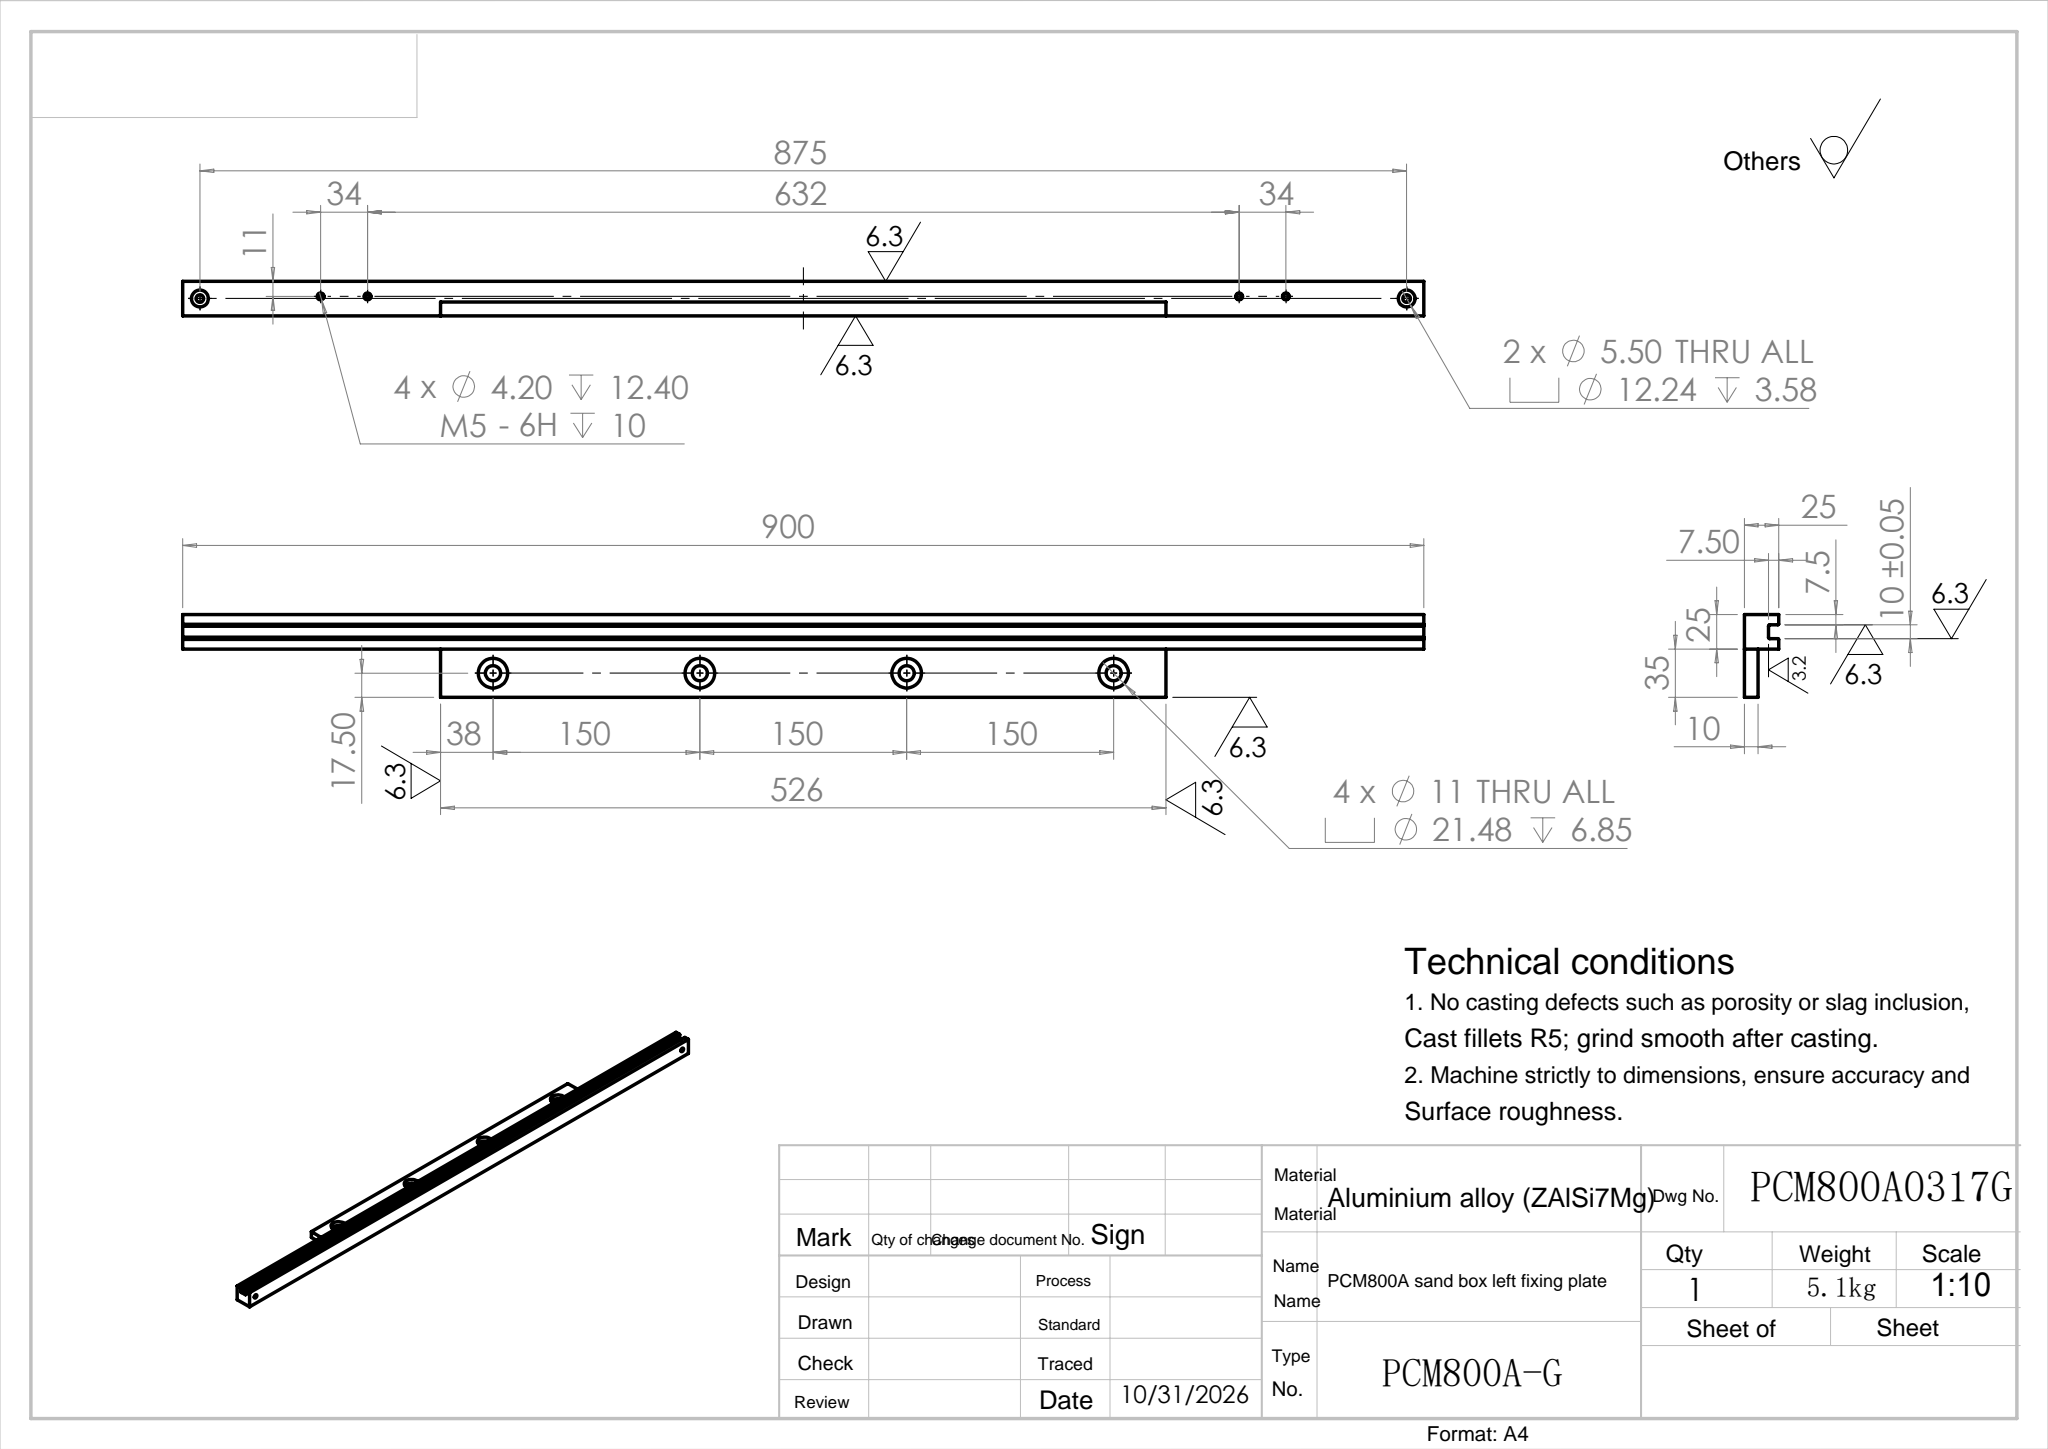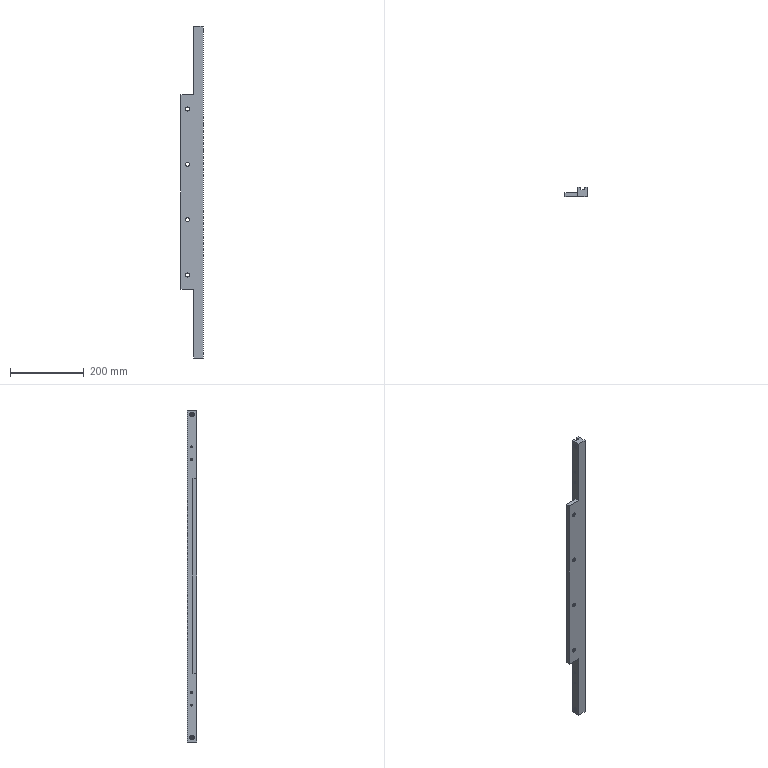Part | SolidWorks | features 3DProfileFeature 3, HoleWzd 3, Boss 1, Chamfer 1, Cut 1, Extrusion 1, LPattern 1 | 1 solid | 76 faces | box 60 x 25 x 900 mm | volume 665333 mm3 | cylinder 42 | plane 26 | cone 8 | commonest cylinder face diameters 4.2 x8 5 x8 11 x8 21.48 x8 5.5 x4 12.24 x4